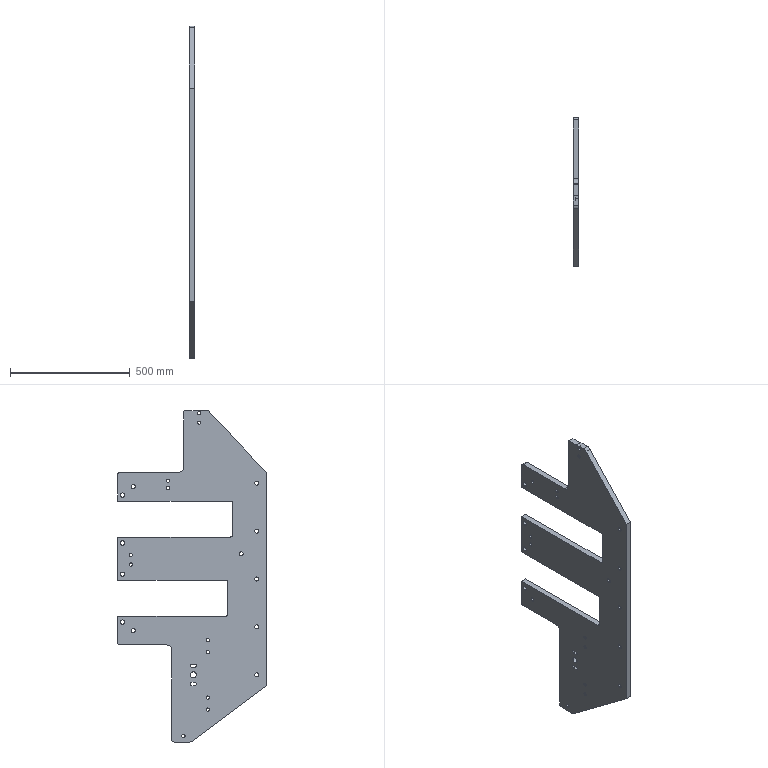Part | SolidWorks | features BaseBody 1 | 1 solid | 147 faces | box 24 x 620 x 1385 mm | volume 11472321 mm3 | cylinder 102 | plane 45 | commonest cylinder face diameters 20 x29 14 x22 17 x16 26 x16 18 x8 13 x4